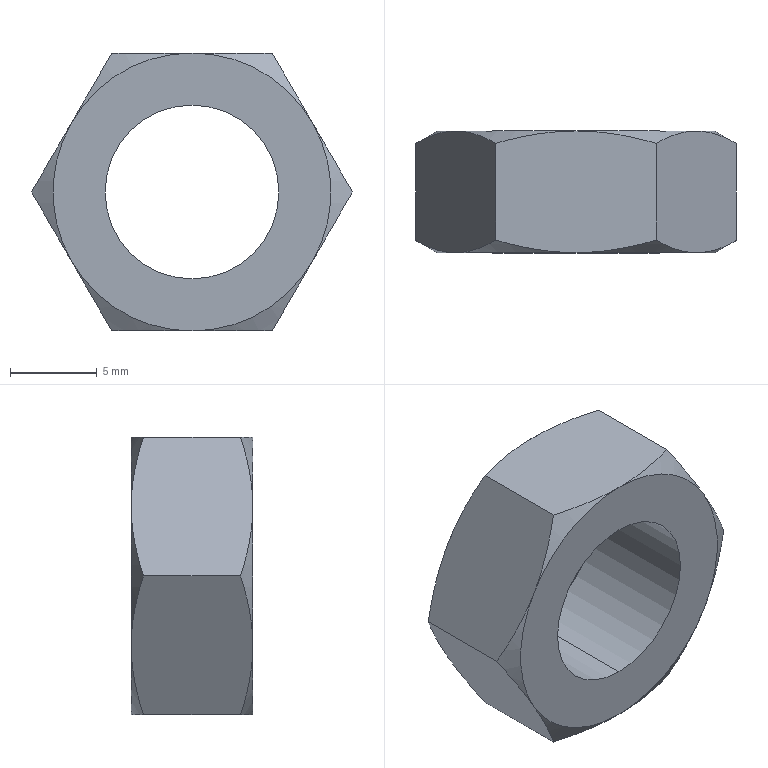Part | 1 solid | 22 faces | box 18.475 x 7 x 16 mm | volume 993.278 mm3 | cone 12 | plane 8 | cylinder 2 | commonest cylinder face diameters 10 x2
STEP:
#1=CARTESIAN_POINT('',(0.,7.,-5.));
#2=VERTEX_POINT('',#1);
#3=CARTESIAN_POINT('',(0.,7.,5.));
#4=VERTEX_POINT('',#3);
#5=CARTESIAN_POINT('',(0.,7.,0.));
#6=DIRECTION('',(0.,1.,0.));
#7=DIRECTION('',(0.,0.,1.));
#8=AXIS2_PLACEMENT_3D('',#5,#6,#7);
#9=CIRCLE('',#8,5.);
#10=EDGE_CURVE('',#2,#4,#9,.T.);
#11=ORIENTED_EDGE('',*,*,#10,.T.);
#12=CARTESIAN_POINT('',(0.,0.,5.));
#13=VERTEX_POINT('',#12);
#14=CARTESIAN_POINT('',(0.,7.,5.));
#15=DIRECTION('',(0.,-1.,0.));
#16=VECTOR('',#15,1000.);
#17=LINE('',#14,#16);
#18=EDGE_CURVE('',#4,#13,#17,.T.);
#19=ORIENTED_EDGE('',*,*,#18,.T.);
#20=CARTESIAN_POINT('',(0.,0.,-5.));
#21=VERTEX_POINT('',#20);
#22=CARTESIAN_POINT('',(0.,0.,0.));
#23=DIRECTION('',(0.,1.,0.));
#24=DIRECTION('',(0.,0.,1.));
#25=AXIS2_PLACEMENT_3D('',#22,#23,#24);
#26=CIRCLE('',#25,5.);
#27=EDGE_CURVE('',#21,#13,#26,.T.);
#28=ORIENTED_EDGE('',*,*,#27,.F.);
#29=CARTESIAN_POINT('',(0.,7.,-5.));
#30=DIRECTION('',(0.,-1.,0.));
#31=VECTOR('',#30,1000.);
#32=LINE('',#29,#31);
#33=EDGE_CURVE('',#2,#21,#32,.T.);
#34=ORIENTED_EDGE('',*,*,#33,.F.);
#35=EDGE_LOOP('',(#11,#19,#28,#34));
#36=FACE_OUTER_BOUND('',#35,.T.);
#37=CARTESIAN_POINT('',(0.,7.,0.));
#38=DIRECTION('',(0.,-1.,0.));
#39=DIRECTION('',(0.,0.,-1.));
#40=AXIS2_PLACEMENT_3D('',#37,#38,#39);
#41=CYLINDRICAL_SURFACE('',#40,5.);
#42=ADVANCED_FACE('',(#36),#41,.F.);
#43=CARTESIAN_POINT('',(9.238,0.7145,0.));
#44=VERTEX_POINT('',#43);
#45=CARTESIAN_POINT('',(6.928,0.,4.));
#46=VERTEX_POINT('',#45);
#47=CARTESIAN_POINT('',(9.238,0.7145,0.));
#48=CARTESIAN_POINT('',(9.041,0.6009,0.341));
#49=CARTESIAN_POINT('',(8.848,0.5005,0.6742));
#50=CARTESIAN_POINT('',(8.563,0.37,1.167));
#51=CARTESIAN_POINT('',(8.469,0.3298,1.331));
#52=CARTESIAN_POINT('',(8.328,0.2745,1.575));
#53=CARTESIAN_POINT('',(8.258,0.2482,1.696));
#54=CARTESIAN_POINT('',(8.188,0.2236,1.818));
#55=CARTESIAN_POINT('',(8.141,0.2077,1.899));
#56=CARTESIAN_POINT('',(8.119,0.2003,1.937));
#57=CARTESIAN_POINT('',(7.997,0.1609,2.148));
#58=CARTESIAN_POINT('',(7.901,0.1333,2.316));
#59=CARTESIAN_POINT('',(7.756,0.09752,2.567));
#60=CARTESIAN_POINT('',(7.708,0.08656,2.65));
#61=CARTESIAN_POINT('',(7.611,0.06657,2.817));
#62=CARTESIAN_POINT('',(7.564,0.05769,2.899));
#63=CARTESIAN_POINT('',(7.318,0.01648,3.325));
#64=CARTESIAN_POINT('',(7.124,0.,3.661));
#65=CARTESIAN_POINT('',(6.928,0.,4.));
#66=B_SPLINE_CURVE_WITH_KNOTS('',3,(#47,#48,#49,#50,#51,#52,#53,#54,#55,#56,#57,#58,#59,#60,#61,#62,#63,#64,#65),.UNSPECIFIED.,.F.,.F.,(4,2,2,1,2,2,2,2,2,4),(0.,0.25,0.375,0.4375,0.4687,0.5,0.625,0.6875,0.75,1.),.UNSPECIFIED.);
#67=EDGE_CURVE('',#44,#46,#66,.T.);
#68=ORIENTED_EDGE('',*,*,#67,.F.);
#69=CARTESIAN_POINT('',(9.238,6.285,0.));
#70=VERTEX_POINT('',#69);
#71=CARTESIAN_POINT('',(9.238,7.,0.));
#72=DIRECTION('',(0.,-1.,0.));
#73=VECTOR('',#72,1000.);
#74=LINE('',#71,#73);
#75=EDGE_CURVE('',#70,#44,#74,.T.);
#76=ORIENTED_EDGE('',*,*,#75,.F.);
#77=CARTESIAN_POINT('',(6.928,7.,4.));
#78=VERTEX_POINT('',#77);
#79=CARTESIAN_POINT('',(6.928,7.,4.));
#80=CARTESIAN_POINT('',(7.026,7.,3.83));
#81=CARTESIAN_POINT('',(7.124,6.996,3.661));
#82=CARTESIAN_POINT('',(7.271,6.983,3.407));
#83=CARTESIAN_POINT('',(7.319,6.978,3.322));
#84=CARTESIAN_POINT('',(7.417,6.966,3.153));
#85=CARTESIAN_POINT('',(7.468,6.959,3.066));
#86=CARTESIAN_POINT('',(7.612,6.934,2.815));
#87=CARTESIAN_POINT('',(7.708,6.914,2.648));
#88=CARTESIAN_POINT('',(7.853,6.878,2.397));
#89=CARTESIAN_POINT('',(7.926,6.859,2.272));
#90=CARTESIAN_POINT('',(7.999,6.837,2.146));
#91=CARTESIAN_POINT('',(8.047,6.823,2.061));
#92=CARTESIAN_POINT('',(8.073,6.815,2.017));
#93=CARTESIAN_POINT('',(8.469,6.686,1.331));
#94=CARTESIAN_POINT('',(8.844,6.512,0.6811));
#95=CARTESIAN_POINT('',(9.238,6.285,0.));
#96=B_SPLINE_CURVE_WITH_KNOTS('',3,(#79,#80,#81,#82,#83,#84,#85,#86,#87,#88,#89,#90,#91,#92,#93,#94,#95),.UNSPECIFIED.,.F.,.F.,(4,2,2,2,2,1,2,2,4),(0.,0.125,0.1875,0.25,0.375,0.4375,0.4687,0.5,1.),.UNSPECIFIED.);
#97=EDGE_CURVE('',#78,#70,#96,.T.);
#98=ORIENTED_EDGE('',*,*,#97,.F.);
#99=CARTESIAN_POINT('',(4.619,6.285,8.));
#100=VERTEX_POINT('',#99);
#101=CARTESIAN_POINT('',(4.619,6.285,8.));
#102=CARTESIAN_POINT('',(4.816,6.399,7.659));
#103=CARTESIAN_POINT('',(5.008,6.499,7.326));
#104=CARTESIAN_POINT('',(5.293,6.63,6.832));
#105=CARTESIAN_POINT('',(5.387,6.67,6.669));
#106=CARTESIAN_POINT('',(5.528,6.725,6.425));
#107=CARTESIAN_POINT('',(5.598,6.752,6.304));
#108=CARTESIAN_POINT('',(5.668,6.776,6.182));
#109=CARTESIAN_POINT('',(5.715,6.792,6.101));
#110=CARTESIAN_POINT('',(5.737,6.8,6.063));
#111=CARTESIAN_POINT('',(5.859,6.839,5.852));
#112=CARTESIAN_POINT('',(5.956,6.867,5.684));
#113=CARTESIAN_POINT('',(6.101,6.902,5.433));
#114=CARTESIAN_POINT('',(6.149,6.913,5.35));
#115=CARTESIAN_POINT('',(6.245,6.933,5.183));
#116=CARTESIAN_POINT('',(6.292,6.942,5.101));
#117=CARTESIAN_POINT('',(6.538,6.984,4.675));
#118=CARTESIAN_POINT('',(6.733,7.,4.339));
#119=CARTESIAN_POINT('',(6.928,7.,4.));
#120=B_SPLINE_CURVE_WITH_KNOTS('',3,(#101,#102,#103,#104,#105,#106,#107,#108,#109,#110,#111,#112,#113,#114,#115,#116,#117,#118,#119),.UNSPECIFIED.,.F.,.F.,(4,2,2,1,2,2,2,2,2,4),(0.,0.25,0.375,0.4375,0.4687,0.5,0.625,0.6875,0.75,1.),.UNSPECIFIED.);
#121=EDGE_CURVE('',#100,#78,#120,.T.);
#122=ORIENTED_EDGE('',*,*,#121,.F.);
#123=CARTESIAN_POINT('',(4.619,0.7145,8.));
#124=VERTEX_POINT('',#123);
#125=CARTESIAN_POINT('',(4.619,7.,8.));
#126=DIRECTION('',(0.,-1.,0.));
#127=VECTOR('',#126,1000.);
#128=LINE('',#125,#127);
#129=EDGE_CURVE('',#100,#124,#128,.T.);
#130=ORIENTED_EDGE('',*,*,#129,.T.);
#131=CARTESIAN_POINT('',(6.928,0.,4.));
#132=CARTESIAN_POINT('',(6.83,0.,4.17));
#133=CARTESIAN_POINT('',(6.732,0.004131,4.339));
#134=CARTESIAN_POINT('',(6.586,0.01652,4.593));
#135=CARTESIAN_POINT('',(6.537,0.02169,4.678));
#136=CARTESIAN_POINT('',(6.439,0.03408,4.847));
#137=CARTESIAN_POINT('',(6.389,0.04148,4.934));
#138=CARTESIAN_POINT('',(6.244,0.06575,5.185));
#139=CARTESIAN_POINT('',(6.148,0.08579,5.352));
#140=CARTESIAN_POINT('',(6.003,0.1216,5.603));
#141=CARTESIAN_POINT('',(5.93,0.141,5.728));
#142=CARTESIAN_POINT('',(5.858,0.1625,5.854));
#143=CARTESIAN_POINT('',(5.809,0.1773,5.939));
#144=CARTESIAN_POINT('',(5.784,0.1853,5.983));
#145=CARTESIAN_POINT('',(5.387,0.3136,6.669));
#146=CARTESIAN_POINT('',(5.012,0.4875,7.319));
#147=CARTESIAN_POINT('',(4.619,0.7145,8.));
#148=B_SPLINE_CURVE_WITH_KNOTS('',3,(#131,#132,#133,#134,#135,#136,#137,#138,#139,#140,#141,#142,#143,#144,#145,#146,#147),.UNSPECIFIED.,.F.,.F.,(4,2,2,2,2,1,2,2,4),(0.,0.125,0.1875,0.25,0.375,0.4375,0.4687,0.5,1.),.UNSPECIFIED.);
#149=EDGE_CURVE('',#46,#124,#148,.T.);
#150=ORIENTED_EDGE('',*,*,#149,.F.);
#151=EDGE_LOOP('',(#68,#76,#98,#122,#130,#150));
#152=FACE_OUTER_BOUND('',#151,.T.);
#153=CARTESIAN_POINT('',(4.619,7.,8.));
#154=DIRECTION('',(-0.866,0.,-0.5));
#155=DIRECTION('',(-0.5,0.,0.866));
#156=AXIS2_PLACEMENT_3D('',#153,#154,#155);
#157=PLANE('',#156);
#158=ADVANCED_FACE('',(#152),#157,.F.);
#159=CARTESIAN_POINT('',(4.619,0.7145,-8.));
#160=VERTEX_POINT('',#159);
#161=CARTESIAN_POINT('',(6.928,0.,-4.));
#162=VERTEX_POINT('',#161);
#163=CARTESIAN_POINT('',(4.619,0.7145,-8.));
#164=CARTESIAN_POINT('',(4.816,0.6009,-7.659));
#165=CARTESIAN_POINT('',(5.008,0.5005,-7.326));
#166=CARTESIAN_POINT('',(5.293,0.37,-6.832));
#167=CARTESIAN_POINT('',(5.387,0.3298,-6.669));
#168=CARTESIAN_POINT('',(5.528,0.2745,-6.425));
#169=CARTESIAN_POINT('',(5.598,0.2482,-6.304));
#170=CARTESIAN_POINT('',(5.668,0.2236,-6.182));
#171=CARTESIAN_POINT('',(5.715,0.2077,-6.101));
#172=CARTESIAN_POINT('',(5.737,0.2003,-6.063));
#173=CARTESIAN_POINT('',(5.859,0.1609,-5.852));
#174=CARTESIAN_POINT('',(5.956,0.1333,-5.684));
#175=CARTESIAN_POINT('',(6.101,0.09752,-5.433));
#176=CARTESIAN_POINT('',(6.149,0.08656,-5.35));
#177=CARTESIAN_POINT('',(6.245,0.06657,-5.183));
#178=CARTESIAN_POINT('',(6.292,0.05769,-5.101));
#179=CARTESIAN_POINT('',(6.538,0.01648,-4.675));
#180=CARTESIAN_POINT('',(6.733,0.,-4.339));
#181=CARTESIAN_POINT('',(6.928,0.,-4.));
#182=B_SPLINE_CURVE_WITH_KNOTS('',3,(#163,#164,#165,#166,#167,#168,#169,#170,#171,#172,#173,#174,#175,#176,#177,#178,#179,#180,#181),.UNSPECIFIED.,.F.,.F.,(4,2,2,1,2,2,2,2,2,4),(0.,0.25,0.375,0.4375,0.4687,0.5,0.625,0.6875,0.75,1.),.UNSPECIFIED.);
#183=EDGE_CURVE('',#160,#162,#182,.T.);
#184=ORIENTED_EDGE('',*,*,#183,.F.);
#185=CARTESIAN_POINT('',(4.619,6.285,-8.));
#186=VERTEX_POINT('',#185);
#187=CARTESIAN_POINT('',(4.619,7.,-8.));
#188=DIRECTION('',(0.,-1.,0.));
#189=VECTOR('',#188,1000.);
#190=LINE('',#187,#189);
#191=EDGE_CURVE('',#186,#160,#190,.T.);
#192=ORIENTED_EDGE('',*,*,#191,.F.);
#193=CARTESIAN_POINT('',(6.928,7.,-4.));
#194=VERTEX_POINT('',#193);
#195=CARTESIAN_POINT('',(6.928,7.,-4.));
#196=CARTESIAN_POINT('',(6.83,7.,-4.17));
#197=CARTESIAN_POINT('',(6.732,6.996,-4.339));
#198=CARTESIAN_POINT('',(6.586,6.983,-4.593));
#199=CARTESIAN_POINT('',(6.537,6.978,-4.678));
#200=CARTESIAN_POINT('',(6.439,6.966,-4.847));
#201=CARTESIAN_POINT('',(6.389,6.959,-4.934));
#202=CARTESIAN_POINT('',(6.244,6.934,-5.185));
#203=CARTESIAN_POINT('',(6.148,6.914,-5.352));
#204=CARTESIAN_POINT('',(6.003,6.878,-5.603));
#205=CARTESIAN_POINT('',(5.93,6.859,-5.728));
#206=CARTESIAN_POINT('',(5.858,6.837,-5.854));
#207=CARTESIAN_POINT('',(5.809,6.823,-5.939));
#208=CARTESIAN_POINT('',(5.784,6.815,-5.983));
#209=CARTESIAN_POINT('',(5.387,6.686,-6.669));
#210=CARTESIAN_POINT('',(5.012,6.512,-7.319));
#211=CARTESIAN_POINT('',(4.619,6.285,-8.));
#212=B_SPLINE_CURVE_WITH_KNOTS('',3,(#195,#196,#197,#198,#199,#200,#201,#202,#203,#204,#205,#206,#207,#208,#209,#210,#211),.UNSPECIFIED.,.F.,.F.,(4,2,2,2,2,1,2,2,4),(0.,0.125,0.1875,0.25,0.375,0.4375,0.4688,0.5,1.),.UNSPECIFIED.);
#213=EDGE_CURVE('',#194,#186,#212,.T.);
#214=ORIENTED_EDGE('',*,*,#213,.F.);
#215=CARTESIAN_POINT('',(9.238,6.285,0.));
#216=CARTESIAN_POINT('',(9.041,6.399,-0.341));
#217=CARTESIAN_POINT('',(8.848,6.499,-0.6742));
#218=CARTESIAN_POINT('',(8.563,6.63,-1.167));
#219=CARTESIAN_POINT('',(8.469,6.67,-1.331));
#220=CARTESIAN_POINT('',(8.328,6.725,-1.575));
#221=CARTESIAN_POINT('',(8.258,6.752,-1.696));
#222=CARTESIAN_POINT('',(8.188,6.776,-1.818));
#223=CARTESIAN_POINT('',(8.141,6.792,-1.899));
#224=CARTESIAN_POINT('',(8.119,6.8,-1.937));
#225=CARTESIAN_POINT('',(7.997,6.839,-2.148));
#226=CARTESIAN_POINT('',(7.901,6.867,-2.316));
#227=CARTESIAN_POINT('',(7.756,6.902,-2.567));
#228=CARTESIAN_POINT('',(7.708,6.913,-2.65));
#229=CARTESIAN_POINT('',(7.611,6.933,-2.817));
#230=CARTESIAN_POINT('',(7.564,6.942,-2.899));
#231=CARTESIAN_POINT('',(7.318,6.984,-3.325));
#232=CARTESIAN_POINT('',(7.124,7.,-3.661));
#233=CARTESIAN_POINT('',(6.928,7.,-4.));
#234=B_SPLINE_CURVE_WITH_KNOTS('',3,(#215,#216,#217,#218,#219,#220,#221,#222,#223,#224,#225,#226,#227,#228,#229,#230,#231,#232,#233),.UNSPECIFIED.,.F.,.F.,(4,2,2,1,2,2,2,2,2,4),(0.,0.25,0.375,0.4375,0.4687,0.5,0.625,0.6875,0.75,1.),.UNSPECIFIED.);
#235=EDGE_CURVE('',#70,#194,#234,.T.);
#236=ORIENTED_EDGE('',*,*,#235,.F.);
#237=ORIENTED_EDGE('',*,*,#75,.T.);
#238=CARTESIAN_POINT('',(6.928,0.,-4.));
#239=CARTESIAN_POINT('',(7.026,0.,-3.83));
#240=CARTESIAN_POINT('',(7.124,0.004131,-3.661));
#241=CARTESIAN_POINT('',(7.271,0.01652,-3.407));
#242=CARTESIAN_POINT('',(7.319,0.02169,-3.322));
#243=CARTESIAN_POINT('',(7.417,0.03408,-3.153));
#244=CARTESIAN_POINT('',(7.468,0.04148,-3.066));
#245=CARTESIAN_POINT('',(7.612,0.06575,-2.815));
#246=CARTESIAN_POINT('',(7.708,0.08579,-2.648));
#247=CARTESIAN_POINT('',(7.853,0.1216,-2.397));
#248=CARTESIAN_POINT('',(7.926,0.141,-2.272));
#249=CARTESIAN_POINT('',(7.999,0.1625,-2.146));
#250=CARTESIAN_POINT('',(8.047,0.1773,-2.061));
#251=CARTESIAN_POINT('',(8.073,0.1853,-2.017));
#252=CARTESIAN_POINT('',(8.469,0.3136,-1.331));
#253=CARTESIAN_POINT('',(8.844,0.4875,-0.6811));
#254=CARTESIAN_POINT('',(9.238,0.7145,0.));
#255=B_SPLINE_CURVE_WITH_KNOTS('',3,(#238,#239,#240,#241,#242,#243,#244,#245,#246,#247,#248,#249,#250,#251,#252,#253,#254),.UNSPECIFIED.,.F.,.F.,(4,2,2,2,2,1,2,2,4),(0.,0.125,0.1875,0.25,0.375,0.4375,0.4688,0.5,1.),.UNSPECIFIED.);
#256=EDGE_CURVE('',#162,#44,#255,.T.);
#257=ORIENTED_EDGE('',*,*,#256,.F.);
#258=EDGE_LOOP('',(#184,#192,#214,#236,#237,#257));
#259=FACE_OUTER_BOUND('',#258,.T.);
#260=CARTESIAN_POINT('',(9.238,7.,0.));
#261=DIRECTION('',(-0.866,0.,0.5));
#262=DIRECTION('',(0.,1.,0.));
#263=AXIS2_PLACEMENT_3D('',#260,#261,#262);
#264=PLANE('',#263);
#265=ADVANCED_FACE('',(#259),#264,.F.);
#266=CARTESIAN_POINT('',(-4.619,0.7145,-8.));
#267=VERTEX_POINT('',#266);
#268=CARTESIAN_POINT('',(0.,0.,-8.));
#269=VERTEX_POINT('',#268);
#270=CARTESIAN_POINT('',(-4.619,0.7145,-8.));
#271=CARTESIAN_POINT('',(-4.224,0.6006,-8.));
#272=CARTESIAN_POINT('',(-3.838,0.5,-8.));
#273=CARTESIAN_POINT('',(-3.267,0.3692,-8.));
#274=CARTESIAN_POINT('',(-3.078,0.329,-8.));
#275=CARTESIAN_POINT('',(-2.796,0.2737,-8.));
#276=CARTESIAN_POINT('',(-2.655,0.2472,-8.));
#277=CARTESIAN_POINT('',(-2.515,0.2227,-8.));
#278=CARTESIAN_POINT('',(-2.421,0.2068,-8.));
#279=CARTESIAN_POINT('',(-2.376,0.1993,-8.));
#280=CARTESIAN_POINT('',(-2.132,0.1601,-8.));
#281=CARTESIAN_POINT('',(-1.939,0.1325,-8.));
#282=CARTESIAN_POINT('',(-1.65,0.09686,-8.));
#283=CARTESIAN_POINT('',(-1.553,0.08594,-8.));
#284=CARTESIAN_POINT('',(-1.36,0.06602,-8.));
#285=CARTESIAN_POINT('',(-1.266,0.05715,-8.));
#286=CARTESIAN_POINT('',(-0.776,0.01633,-8.));
#287=CARTESIAN_POINT('',(-0.3895,0.,-8.));
#288=CARTESIAN_POINT('',(0.,0.,-8.));
#289=B_SPLINE_CURVE_WITH_KNOTS('',3,(#270,#271,#272,#273,#274,#275,#276,#277,#278,#279,#280,#281,#282,#283,#284,#285,#286,#287,#288),.UNSPECIFIED.,.F.,.F.,(4,2,2,1,2,2,2,2,2,4),(0.,0.25,0.375,0.4375,0.4687,0.5,0.625,0.6875,0.75,1.),.UNSPECIFIED.);
#290=EDGE_CURVE('',#267,#269,#289,.T.);
#291=ORIENTED_EDGE('',*,*,#290,.F.);
#292=CARTESIAN_POINT('',(-4.619,6.285,-8.));
#293=VERTEX_POINT('',#292);
#294=CARTESIAN_POINT('',(-4.619,7.,-8.));
#295=DIRECTION('',(0.,-1.,0.));
#296=VECTOR('',#295,1000.);
#297=LINE('',#294,#296);
#298=EDGE_CURVE('',#293,#267,#297,.T.);
#299=ORIENTED_EDGE('',*,*,#298,.F.);
#300=CARTESIAN_POINT('',(0.,7.,-8.));
#301=VERTEX_POINT('',#300);
#302=CARTESIAN_POINT('',(0.,7.,-8.));
#303=CARTESIAN_POINT('',(-0.1947,7.,-8.));
#304=CARTESIAN_POINT('',(-0.3887,6.996,-8.));
#305=CARTESIAN_POINT('',(-0.6801,6.984,-8.));
#306=CARTESIAN_POINT('',(-0.7773,6.979,-8.));
#307=CARTESIAN_POINT('',(-0.9721,6.966,-8.));
#308=CARTESIAN_POINT('',(-1.071,6.959,-8.));
#309=CARTESIAN_POINT('',(-1.36,6.935,-8.));
#310=CARTESIAN_POINT('',(-1.553,6.915,-8.));
#311=CARTESIAN_POINT('',(-1.842,6.879,-8.));
#312=CARTESIAN_POINT('',(-1.987,6.86,-8.));
#313=CARTESIAN_POINT('',(-2.133,6.839,-8.));
#314=CARTESIAN_POINT('',(-2.23,6.824,-8.));
#315=CARTESIAN_POINT('',(-2.28,6.816,-8.));
#316=CARTESIAN_POINT('',(-3.076,6.688,-8.));
#317=CARTESIAN_POINT('',(-3.829,6.513,-8.));
#318=CARTESIAN_POINT('',(-4.619,6.285,-8.));
#319=B_SPLINE_CURVE_WITH_KNOTS('',3,(#302,#303,#304,#305,#306,#307,#308,#309,#310,#311,#312,#313,#314,#315,#316,#317,#318),.UNSPECIFIED.,.F.,.F.,(4,2,2,2,2,1,2,2,4),(0.,0.125,0.1875,0.25,0.375,0.4375,0.4687,0.5,1.),.UNSPECIFIED.);
#320=EDGE_CURVE('',#301,#293,#319,.T.);
#321=ORIENTED_EDGE('',*,*,#320,.F.);
#322=CARTESIAN_POINT('',(4.619,6.285,-8.));
#323=CARTESIAN_POINT('',(4.227,6.399,-8.));
#324=CARTESIAN_POINT('',(3.844,6.498,-8.));
#325=CARTESIAN_POINT('',(3.277,6.629,-8.));
#326=CARTESIAN_POINT('',(3.09,6.669,-8.));
#327=CARTESIAN_POINT('',(2.81,6.724,-8.));
#328=CARTESIAN_POINT('',(2.67,6.75,-8.));
#329=CARTESIAN_POINT('',(2.507,6.779,-8.));
#330=CARTESIAN_POINT('',(2.437,6.79,-8.));
#331=CARTESIAN_POINT('',(2.391,6.798,-8.));
#332=CARTESIAN_POINT('',(2.369,6.802,-8.));
#333=CARTESIAN_POINT('',(2.149,6.838,-8.));
#334=CARTESIAN_POINT('',(1.954,6.865,-8.));
#335=CARTESIAN_POINT('',(1.662,6.902,-8.));
#336=CARTESIAN_POINT('',(1.565,6.913,-8.));
#337=CARTESIAN_POINT('',(1.371,6.933,-8.));
#338=CARTESIAN_POINT('',(1.275,6.942,-8.));
#339=CARTESIAN_POINT('',(0.7811,6.983,-8.));
#340=CARTESIAN_POINT('',(0.3917,7.,-8.));
#341=CARTESIAN_POINT('',(0.,7.,-8.));
#342=B_SPLINE_CURVE_WITH_KNOTS('',3,(#322,#323,#324,#325,#326,#327,#328,#329,#330,#331,#332,#333,#334,#335,#336,#337,#338,#339,#340,#341),.UNSPECIFIED.,.F.,.F.,(4,2,2,1,1,2,2,2,2,2,4),(0.,0.25,0.375,0.4375,0.4688,0.4844,0.5,0.625,0.6875,0.75,1.),.UNSPECIFIED.);
#343=EDGE_CURVE('',#186,#301,#342,.T.);
#344=ORIENTED_EDGE('',*,*,#343,.F.);
#345=ORIENTED_EDGE('',*,*,#191,.T.);
#346=CARTESIAN_POINT('',(0.,0.,-8.));
#347=CARTESIAN_POINT('',(0.1958,0.,-8.));
#348=CARTESIAN_POINT('',(0.3911,0.00415,-8.));
#349=CARTESIAN_POINT('',(0.6847,0.0166,-8.));
#350=CARTESIAN_POINT('',(0.7826,0.02179,-8.));
#351=CARTESIAN_POINT('',(0.9791,0.03423,-8.));
#352=CARTESIAN_POINT('',(1.079,0.04163,-8.));
#353=CARTESIAN_POINT('',(1.371,0.06613,-8.));
#354=CARTESIAN_POINT('',(1.565,0.08634,-8.));
#355=CARTESIAN_POINT('',(1.857,0.1225,-8.));
#356=CARTESIAN_POINT('',(2.002,0.142,-8.));
#357=CARTESIAN_POINT('',(2.173,0.1673,-8.));
#358=CARTESIAN_POINT('',(2.247,0.1786,-8.));
#359=CARTESIAN_POINT('',(2.295,0.1864,-8.));
#360=CARTESIAN_POINT('',(2.321,0.1905,-8.));
#361=CARTESIAN_POINT('',(3.088,0.3149,-8.));
#362=CARTESIAN_POINT('',(3.835,0.4884,-8.));
#363=CARTESIAN_POINT('',(4.619,0.7145,-8.));
#364=B_SPLINE_CURVE_WITH_KNOTS('',3,(#346,#347,#348,#349,#350,#351,#352,#353,#354,#355,#356,#357,#358,#359,#360,#361,#362,#363),.UNSPECIFIED.,.F.,.F.,(4,2,2,2,2,1,1,2,2,4),(0.,0.125,0.1875,0.25,0.375,0.4375,0.4688,0.4844,0.5,1.),.UNSPECIFIED.);
#365=EDGE_CURVE('',#269,#160,#364,.T.);
#366=ORIENTED_EDGE('',*,*,#365,.F.);
#367=EDGE_LOOP('',(#291,#299,#321,#344,#345,#366));
#368=FACE_OUTER_BOUND('',#367,.T.);
#369=CARTESIAN_POINT('',(4.619,7.,-8.));
#370=DIRECTION('',(0.,0.,1.));
#371=DIRECTION('',(1.,0.,0.));
#372=AXIS2_PLACEMENT_3D('',#369,#370,#371);
#373=PLANE('',#372);
#374=ADVANCED_FACE('',(#368),#373,.F.);
#375=CARTESIAN_POINT('',(-9.238,0.7145,0.));
#376=VERTEX_POINT('',#375);
#377=CARTESIAN_POINT('',(-6.928,0.,-4.));
#378=VERTEX_POINT('',#377);
#379=CARTESIAN_POINT('',(-9.238,0.7145,0.));
#380=CARTESIAN_POINT('',(-9.041,0.6009,-0.341));
#381=CARTESIAN_POINT('',(-8.848,0.5005,-0.6742));
#382=CARTESIAN_POINT('',(-8.563,0.37,-1.167));
#383=CARTESIAN_POINT('',(-8.469,0.3298,-1.331));
#384=CARTESIAN_POINT('',(-8.328,0.2745,-1.575));
#385=CARTESIAN_POINT('',(-8.258,0.2482,-1.696));
#386=CARTESIAN_POINT('',(-8.188,0.2236,-1.818));
#387=CARTESIAN_POINT('',(-8.141,0.2077,-1.899));
#388=CARTESIAN_POINT('',(-8.119,0.2003,-1.937));
#389=CARTESIAN_POINT('',(-7.997,0.1609,-2.148));
#390=CARTESIAN_POINT('',(-7.901,0.1333,-2.316));
#391=CARTESIAN_POINT('',(-7.756,0.09752,-2.567));
#392=CARTESIAN_POINT('',(-7.708,0.08656,-2.65));
#393=CARTESIAN_POINT('',(-7.611,0.06657,-2.817));
#394=CARTESIAN_POINT('',(-7.564,0.05769,-2.899));
#395=CARTESIAN_POINT('',(-7.318,0.01648,-3.325));
#396=CARTESIAN_POINT('',(-7.124,0.,-3.661));
#397=CARTESIAN_POINT('',(-6.928,0.,-4.));
#398=B_SPLINE_CURVE_WITH_KNOTS('',3,(#379,#380,#381,#382,#383,#384,#385,#386,#387,#388,#389,#390,#391,#392,#393,#394,#395,#396,#397),.UNSPECIFIED.,.F.,.F.,(4,2,2,1,2,2,2,2,2,4),(0.,0.25,0.375,0.4375,0.4688,0.5,0.625,0.6875,0.75,1.),.UNSPECIFIED.);
#399=EDGE_CURVE('',#376,#378,#398,.T.);
#400=ORIENTED_EDGE('',*,*,#399,.F.);
#401=CARTESIAN_POINT('',(-9.238,6.285,0.));
#402=VERTEX_POINT('',#401);
#403=CARTESIAN_POINT('',(-9.238,7.,0.));
#404=DIRECTION('',(0.,-1.,0.));
#405=VECTOR('',#404,1000.);
#406=LINE('',#403,#405);
#407=EDGE_CURVE('',#402,#376,#406,.T.);
#408=ORIENTED_EDGE('',*,*,#407,.F.);
#409=CARTESIAN_POINT('',(-6.928,7.,-4.));
#410=VERTEX_POINT('',#409);
#411=CARTESIAN_POINT('',(-6.928,7.,-4.));
#412=CARTESIAN_POINT('',(-7.026,7.,-3.83));
#413=CARTESIAN_POINT('',(-7.124,6.996,-3.661));
#414=CARTESIAN_POINT('',(-7.271,6.983,-3.407));
#415=CARTESIAN_POINT('',(-7.319,6.978,-3.322));
#416=CARTESIAN_POINT('',(-7.417,6.966,-3.153));
#417=CARTESIAN_POINT('',(-7.468,6.959,-3.066));
#418=CARTESIAN_POINT('',(-7.612,6.934,-2.815));
#419=CARTESIAN_POINT('',(-7.708,6.914,-2.648));
#420=CARTESIAN_POINT('',(-7.853,6.878,-2.397));
#421=CARTESIAN_POINT('',(-7.926,6.859,-2.272));
#422=CARTESIAN_POINT('',(-7.999,6.837,-2.146));
#423=CARTESIAN_POINT('',(-8.047,6.823,-2.061));
#424=CARTESIAN_POINT('',(-8.073,6.815,-2.017));
#425=CARTESIAN_POINT('',(-8.469,6.686,-1.331));
#426=CARTESIAN_POINT('',(-8.844,6.512,-0.6811));
#427=CARTESIAN_POINT('',(-9.238,6.285,0.));
#428=B_SPLINE_CURVE_WITH_KNOTS('',3,(#411,#412,#413,#414,#415,#416,#417,#418,#419,#420,#421,#422,#423,#424,#425,#426,#427),.UNSPECIFIED.,.F.,.F.,(4,2,2,2,2,1,2,2,4),(0.,0.125,0.1875,0.25,0.375,0.4375,0.4687,0.5,1.),.UNSPECIFIED.);
#429=EDGE_CURVE('',#410,#402,#428,.T.);
#430=ORIENTED_EDGE('',*,*,#429,.F.);
#431=CARTESIAN_POINT('',(-4.619,6.285,-8.));
#432=CARTESIAN_POINT('',(-4.816,6.399,-7.659));
#433=CARTESIAN_POINT('',(-5.008,6.499,-7.326));
#434=CARTESIAN_POINT('',(-5.293,6.63,-6.832));
#435=CARTESIAN_POINT('',(-5.387,6.67,-6.669));
#436=CARTESIAN_POINT('',(-5.528,6.725,-6.425));
#437=CARTESIAN_POINT('',(-5.598,6.752,-6.304));
#438=CARTESIAN_POINT('',(-5.668,6.776,-6.182));
#439=CARTESIAN_POINT('',(-5.715,6.792,-6.101));
#440=CARTESIAN_POINT('',(-5.737,6.8,-6.063));
#441=CARTESIAN_POINT('',(-5.859,6.839,-5.852));
#442=CARTESIAN_POINT('',(-5.956,6.867,-5.684));
#443=CARTESIAN_POINT('',(-6.101,6.902,-5.433));
#444=CARTESIAN_POINT('',(-6.149,6.913,-5.35));
#445=CARTESIAN_POINT('',(-6.245,6.933,-5.183));
#446=CARTESIAN_POINT('',(-6.292,6.942,-5.101));
#447=CARTESIAN_POINT('',(-6.538,6.984,-4.675));
#448=CARTESIAN_POINT('',(-6.733,7.,-4.339));
#449=CARTESIAN_POINT('',(-6.928,7.,-4.));
#450=B_SPLINE_CURVE_WITH_KNOTS('',3,(#431,#432,#433,#434,#435,#436,#437,#438,#439,#440,#441,#442,#443,#444,#445,#446,#447,#448,#449),.UNSPECIFIED.,.F.,.F.,(4,2,2,1,2,2,2,2,2,4),(0.,0.25,0.375,0.4375,0.4688,0.5,0.625,0.6875,0.75,1.),.UNSPECIFIED.);
#451=EDGE_CURVE('',#293,#410,#450,.T.);
#452=ORIENTED_EDGE('',*,*,#451,.F.);
#453=ORIENTED_EDGE('',*,*,#298,.T.);
#454=CARTESIAN_POINT('',(-6.928,0.,-4.));
#455=CARTESIAN_POINT('',(-6.83,0.,-4.17));
#456=CARTESIAN_POINT('',(-6.732,0.004131,-4.339));
#457=CARTESIAN_POINT('',(-6.586,0.01652,-4.593));
#458=CARTESIAN_POINT('',(-6.537,0.02169,-4.678));
#459=CARTESIAN_POINT('',(-6.439,0.03408,-4.847));
#460=CARTESIAN_POINT('',(-6.389,0.04148,-4.934));
#461=CARTESIAN_POINT('',(-6.244,0.06575,-5.185));
#462=CARTESIAN_POINT('',(-6.148,0.08579,-5.352));
#463=CARTESIAN_POINT('',(-6.003,0.1216,-5.603));
#464=CARTESIAN_POINT('',(-5.93,0.141,-5.728));
#465=CARTESIAN_POINT('',(-5.858,0.1625,-5.854));
#466=CARTESIAN_POINT('',(-5.809,0.1773,-5.939));
#467=CARTESIAN_POINT('',(-5.784,0.1853,-5.983));
#468=CARTESIAN_POINT('',(-5.387,0.3136,-6.669));
#469=CARTESIAN_POINT('',(-5.012,0.4875,-7.319));
#470=CARTESIAN_POINT('',(-4.619,0.7145,-8.));
#471=B_SPLINE_CURVE_WITH_KNOTS('',3,(#454,#455,#456,#457,#458,#459,#460,#461,#462,#463,#464,#465,#466,#467,#468,#469,#470),.UNSPECIFIED.,.F.,.F.,(4,2,2,2,2,1,2,2,4),(0.,0.125,0.1875,0.25,0.375,0.4375,0.4687,0.5,1.),.UNSPECIFIED.);
#472=EDGE_CURVE('',#378,#267,#471,.T.);
#473=ORIENTED_EDGE('',*,*,#472,.F.);
#474=EDGE_LOOP('',(#400,#408,#430,#452,#453,#473));
#475=FACE_OUTER_BOUND('',#474,.T.);
#476=CARTESIAN_POINT('',(-4.619,7.,-8.));
#477=DIRECTION('',(0.866,0.,0.5));
#478=DIRECTION('',(0.,-1.,0.));
#479=AXIS2_PLACEMENT_3D('',#476,#477,#478);
#480=PLANE('',#479);
#481=ADVANCED_FACE('',(#475),#480,.F.);
#482=CARTESIAN_POINT('',(-4.619,0.7145,8.));
#483=VERTEX_POINT('',#482);
#484=CARTESIAN_POINT('',(-6.928,0.,4.));
#485=VERTEX_POINT('',#484);
#486=CARTESIAN_POINT('',(-4.619,0.7145,8.));
#487=CARTESIAN_POINT('',(-4.816,0.6009,7.659));
#488=CARTESIAN_POINT('',(-5.008,0.5005,7.326));
#489=CARTESIAN_POINT('',(-5.293,0.37,6.832));
#490=CARTESIAN_POINT('',(-5.387,0.3298,6.669));
#491=CARTESIAN_POINT('',(-5.528,0.2745,6.425));
#492=CARTESIAN_POINT('',(-5.598,0.2482,6.304));
#493=CARTESIAN_POINT('',(-5.668,0.2236,6.182));
#494=CARTESIAN_POINT('',(-5.715,0.2077,6.101));
#495=CARTESIAN_POINT('',(-5.737,0.2003,6.063));
#496=CARTESIAN_POINT('',(-5.859,0.1609,5.852));
#497=CARTESIAN_POINT('',(-5.956,0.1333,5.684));
#498=CARTESIAN_POINT('',(-6.101,0.09752,5.433));
#499=CARTESIAN_POINT('',(-6.149,0.08656,5.35));
#500=CARTESIAN_POINT('',(-6.245,0.06657,5.183));
#501=CARTESIAN_POINT('',(-6.292,0.05769,5.101));
#502=CARTESIAN_POINT('',(-6.538,0.01648,4.675));
#503=CARTESIAN_POINT('',(-6.733,0.,4.339));
#504=CARTESIAN_POINT('',(-6.928,0.,4.));
#505=B_SPLINE_CURVE_WITH_KNOTS('',3,(#486,#487,#488,#489,#490,#491,#492,#493,#494,#495,#496,#497,#498,#499,#500,#501,#502,#503,#504),.UNSPECIFIED.,.F.,.F.,(4,2,2,1,2,2,2,2,2,4),(0.,0.25,0.375,0.4375,0.4688,0.5,0.625,0.6875,0.75,1.),.UNSPECIFIED.);
#506=EDGE_CURVE('',#483,#485,#505,.T.);
#507=ORIENTED_EDGE('',*,*,#506,.F.);
#508=CARTESIAN_POINT('',(-4.619,6.285,8.));
#509=VERTEX_POINT('',#508);
#510=CARTESIAN_POINT('',(-4.619,7.,8.));
#511=DIRECTION('',(0.,-1.,0.));
#512=VECTOR('',#511,1000.);
#513=LINE('',#510,#512);
#514=EDGE_CURVE('',#509,#483,#513,.T.);
#515=ORIENTED_EDGE('',*,*,#514,.F.);
#516=CARTESIAN_POINT('',(-6.928,7.,4.));
#517=VERTEX_POINT('',#516);
#518=CARTESIAN_POINT('',(-6.928,7.,4.));
#519=CARTESIAN_POINT('',(-6.83,7.,4.17));
#520=CARTESIAN_POINT('',(-6.732,6.996,4.339));
#521=CARTESIAN_POINT('',(-6.586,6.983,4.593));
#522=CARTESIAN_POINT('',(-6.537,6.978,4.678));
#523=CARTESIAN_POINT('',(-6.439,6.966,4.847));
#524=CARTESIAN_POINT('',(-6.389,6.959,4.934));
#525=CARTESIAN_POINT('',(-6.244,6.934,5.185));
#526=CARTESIAN_POINT('',(-6.148,6.914,5.352));
#527=CARTESIAN_POINT('',(-6.003,6.878,5.603));
#528=CARTESIAN_POINT('',(-5.93,6.859,5.728));
#529=CARTESIAN_POINT('',(-5.858,6.837,5.854));
#530=CARTESIAN_POINT('',(-5.809,6.823,5.939));
#531=CARTESIAN_POINT('',(-5.784,6.815,5.983));
#532=CARTESIAN_POINT('',(-5.387,6.686,6.669));
#533=CARTESIAN_POINT('',(-5.012,6.512,7.319));
#534=CARTESIAN_POINT('',(-4.619,6.285,8.));
#535=B_SPLINE_CURVE_WITH_KNOTS('',3,(#518,#519,#520,#521,#522,#523,#524,#525,#526,#527,#528,#529,#530,#531,#532,#533,#534),.UNSPECIFIED.,.F.,.F.,(4,2,2,2,2,1,2,2,4),(0.,0.125,0.1875,0.25,0.375,0.4375,0.4687,0.5,1.),.UNSPECIFIED.);
#536=EDGE_CURVE('',#517,#509,#535,.T.);
#537=ORIENTED_EDGE('',*,*,#536,.F.);
#538=CARTESIAN_POINT('',(-9.238,6.285,0.));
#539=CARTESIAN_POINT('',(-9.041,6.399,0.341));
#540=CARTESIAN_POINT('',(-8.848,6.499,0.6742));
#541=CARTESIAN_POINT('',(-8.563,6.63,1.167));
#542=CARTESIAN_POINT('',(-8.469,6.67,1.331));
#543=CARTESIAN_POINT('',(-8.328,6.725,1.575));
#544=CARTESIAN_POINT('',(-8.258,6.752,1.696));
#545=CARTESIAN_POINT('',(-8.188,6.776,1.818));
#546=CARTESIAN_POINT('',(-8.141,6.792,1.899));
#547=CARTESIAN_POINT('',(-8.119,6.8,1.937));
#548=CARTESIAN_POINT('',(-7.997,6.839,2.148));
#549=CARTESIAN_POINT('',(-7.901,6.867,2.316));
#550=CARTESIAN_POINT('',(-7.756,6.902,2.567));
#551=CARTESIAN_POINT('',(-7.708,6.913,2.65));
#552=CARTESIAN_POINT('',(-7.611,6.933,2.817));
#553=CARTESIAN_POINT('',(-7.564,6.942,2.899));
#554=CARTESIAN_POINT('',(-7.318,6.984,3.325));
#555=CARTESIAN_POINT('',(-7.124,7.,3.661));
#556=CARTESIAN_POINT('',(-6.928,7.,4.));
#557=B_SPLINE_CURVE_WITH_KNOTS('',3,(#538,#539,#540,#541,#542,#543,#544,#545,#546,#547,#548,#549,#550,#551,#552,#553,#554,#555,#556),.UNSPECIFIED.,.F.,.F.,(4,2,2,1,2,2,2,2,2,4),(0.,0.25,0.375,0.4375,0.4687,0.5,0.625,0.6875,0.75,1.),.UNSPECIFIED.);
#558=EDGE_CURVE('',#402,#517,#557,.T.);
#559=ORIENTED_EDGE('',*,*,#558,.F.);
#560=ORIENTED_EDGE('',*,*,#407,.T.);
#561=CARTESIAN_POINT('',(-6.928,0.,4.));
#562=CARTESIAN_POINT('',(-7.026,0.,3.83));
#563=CARTESIAN_POINT('',(-7.124,0.004131,3.661));
#564=CARTESIAN_POINT('',(-7.271,0.01652,3.407));
#565=CARTESIAN_POINT('',(-7.319,0.02169,3.322));
#566=CARTESIAN_POINT('',(-7.417,0.03408,3.153));
#567=CARTESIAN_POINT('',(-7.468,0.04148,3.066));
#568=CARTESIAN_POINT('',(-7.612,0.06575,2.815));
#569=CARTESIAN_POINT('',(-7.708,0.08579,2.648));
#570=CARTESIAN_POINT('',(-7.853,0.1216,2.397));
#571=CARTESIAN_POINT('',(-7.926,0.141,2.272));
#572=CARTESIAN_POINT('',(-7.999,0.1625,2.146));
#573=CARTESIAN_POINT('',(-8.047,0.1773,2.061));
#574=CARTESIAN_POINT('',(-8.073,0.1853,2.017));
#575=CARTESIAN_POINT('',(-8.469,0.3136,1.331));
#576=CARTESIAN_POINT('',(-8.844,0.4875,0.6811));
#577=CARTESIAN_POINT('',(-9.238,0.7145,0.));
#578=B_SPLINE_CURVE_WITH_KNOTS('',3,(#561,#562,#563,#564,#565,#566,#567,#568,#569,#570,#571,#572,#573,#574,#575,#576,#577),.UNSPECIFIED.,.F.,.F.,(4,2,2,2,2,1,2,2,4),(0.,0.125,0.1875,0.25,0.375,0.4375,0.4688,0.5,1.),.UNSPECIFIED.);
#579=EDGE_CURVE('',#485,#376,#578,.T.);
#580=ORIENTED_EDGE('',*,*,#579,.F.);
#581=EDGE_LOOP('',(#507,#515,#537,#559,#560,#580));
#582=FACE_OUTER_BOUND('',#581,.T.);
#583=CARTESIAN_POINT('',(-9.238,7.,0.));
#584=DIRECTION('',(0.866,0.,-0.5));
#585=DIRECTION('',(0.,-1.,0.));
#586=AXIS2_PLACEMENT_3D('',#583,#584,#585);
#587=PLANE('',#586);
#588=ADVANCED_FACE('',(#582),#587,.F.);
#589=CARTESIAN_POINT('',(0.,0.,8.));
#590=VERTEX_POINT('',#589);
#591=CARTESIAN_POINT('',(4.619,0.7145,8.));
#592=CARTESIAN_POINT('',(4.227,0.6015,8.));
#593=CARTESIAN_POINT('',(3.844,0.5016,8.));
#594=CARTESIAN_POINT('',(3.277,0.3715,8.));
#595=CARTESIAN_POINT('',(3.09,0.3314,8.));
#596=CARTESIAN_POINT('',(2.81,0.2763,8.));
#597=CARTESIAN_POINT('',(2.67,0.2499,8.));
#598=CARTESIAN_POINT('',(2.507,0.2214,8.));
#599=CARTESIAN_POINT('',(2.437,0.2096,8.));
#600=CARTESIAN_POINT('',(2.391,0.2018,8.));
#601=CARTESIAN_POINT('',(2.369,0.1982,8.));
#602=CARTESIAN_POINT('',(2.149,0.1624,8.));
#603=CARTESIAN_POINT('',(1.954,0.1345,8.));
#604=CARTESIAN_POINT('',(1.662,0.09839,8.));
#605=CARTESIAN_POINT('',(1.565,0.08732,8.));
#606=CARTESIAN_POINT('',(1.371,0.06711,8.));
#607=CARTESIAN_POINT('',(1.275,0.05809,8.));
#608=CARTESIAN_POINT('',(0.7811,0.0166,8.));
#609=CARTESIAN_POINT('',(0.3917,0.,8.));
#610=CARTESIAN_POINT('',(0.,0.,8.));
#611=B_SPLINE_CURVE_WITH_KNOTS('',3,(#591,#592,#593,#594,#595,#596,#597,#598,#599,#600,#601,#602,#603,#604,#605,#606,#607,#608,#609,#610),.UNSPECIFIED.,.F.,.F.,(4,2,2,1,1,2,2,2,2,2,4),(0.,0.25,0.375,0.4375,0.4687,0.4844,0.5,0.625,0.6875,0.75,1.),.UNSPECIFIED.);
#612=EDGE_CURVE('',#124,#590,#611,.T.);
#613=ORIENTED_EDGE('',*,*,#612,.F.);
#614=ORIENTED_EDGE('',*,*,#129,.F.);
#615=CARTESIAN_POINT('',(0.,7.,8.));
#616=VERTEX_POINT('',#615);
#617=CARTESIAN_POINT('',(0.,7.,8.));
#618=CARTESIAN_POINT('',(0.1958,7.,8.));
#619=CARTESIAN_POINT('',(0.3911,6.996,8.));
#620=CARTESIAN_POINT('',(0.6847,6.983,8.));
#621=CARTESIAN_POINT('',(0.7826,6.978,8.));
#622=CARTESIAN_POINT('',(0.9791,6.966,8.));
#623=CARTESIAN_POINT('',(1.079,6.958,8.));
#624=CARTESIAN_POINT('',(1.371,6.934,8.));
#625=CARTESIAN_POINT('',(1.565,6.914,8.));
#626=CARTESIAN_POINT('',(1.857,6.878,8.));
#627=CARTESIAN_POINT('',(2.002,6.858,8.));
#628=CARTESIAN_POINT('',(2.173,6.833,8.));
#629=CARTESIAN_POINT('',(2.247,6.821,8.));
#630=CARTESIAN_POINT('',(2.295,6.814,8.));
#631=CARTESIAN_POINT('',(2.321,6.81,8.));
#632=CARTESIAN_POINT('',(3.088,6.685,8.));
#633=CARTESIAN_POINT('',(3.835,6.512,8.));
#634=CARTESIAN_POINT('',(4.619,6.285,8.));
#635=B_SPLINE_CURVE_WITH_KNOTS('',3,(#617,#618,#619,#620,#621,#622,#623,#624,#625,#626,#627,#628,#629,#630,#631,#632,#633,#634),.UNSPECIFIED.,.F.,.F.,(4,2,2,2,2,1,1,2,2,4),(0.,0.125,0.1875,0.25,0.375,0.4375,0.4687,0.4844,0.5,1.),.UNSPECIFIED.);
#636=EDGE_CURVE('',#616,#100,#635,.T.);
#637=ORIENTED_EDGE('',*,*,#636,.F.);
#638=CARTESIAN_POINT('',(-4.619,6.285,8.));
#639=CARTESIAN_POINT('',(-4.224,6.399,8.));
#640=CARTESIAN_POINT('',(-3.838,6.5,8.));
#641=CARTESIAN_POINT('',(-3.267,6.631,8.));
#642=CARTESIAN_POINT('',(-3.078,6.671,8.));
#643=CARTESIAN_POINT('',(-2.796,6.726,8.));
#644=CARTESIAN_POINT('',(-2.655,6.753,8.));
#645=CARTESIAN_POINT('',(-2.515,6.777,8.));
#646=CARTESIAN_POINT('',(-2.421,6.793,8.));
#647=CARTESIAN_POINT('',(-2.376,6.801,8.));
#648=CARTESIAN_POINT('',(-2.132,6.84,8.));
#649=CARTESIAN_POINT('',(-1.939,6.868,8.));
#650=CARTESIAN_POINT('',(-1.65,6.903,8.));
#651=CARTESIAN_POINT('',(-1.553,6.914,8.));
#652=CARTESIAN_POINT('',(-1.36,6.934,8.));
#653=CARTESIAN_POINT('',(-1.266,6.943,8.));
#654=CARTESIAN_POINT('',(-0.776,6.984,8.));
#655=CARTESIAN_POINT('',(-0.3895,7.,8.));
#656=CARTESIAN_POINT('',(0.,7.,8.));
#657=B_SPLINE_CURVE_WITH_KNOTS('',3,(#638,#639,#640,#641,#642,#643,#644,#645,#646,#647,#648,#649,#650,#651,#652,#653,#654,#655,#656),.UNSPECIFIED.,.F.,.F.,(4,2,2,1,2,2,2,2,2,4),(0.,0.25,0.375,0.4375,0.4688,0.5,0.625,0.6875,0.75,1.),.UNSPECIFIED.);
#658=EDGE_CURVE('',#509,#616,#657,.T.);
#659=ORIENTED_EDGE('',*,*,#658,.F.);
#660=ORIENTED_EDGE('',*,*,#514,.T.);
#661=CARTESIAN_POINT('',(0.,0.,8.));
#662=CARTESIAN_POINT('',(-0.1947,0.,8.));
#663=CARTESIAN_POINT('',(-0.3887,0.004082,8.));
#664=CARTESIAN_POINT('',(-0.6801,0.01633,8.));
#665=CARTESIAN_POINT('',(-0.7773,0.02143,8.));
#666=CARTESIAN_POINT('',(-0.9721,0.03368,8.));
#667=CARTESIAN_POINT('',(-1.071,0.04094,8.));
#668=CARTESIAN_POINT('',(-1.36,0.06506,8.));
#669=CARTESIAN_POINT('',(-1.553,0.08498,8.));
#670=CARTESIAN_POINT('',(-1.842,0.1206,8.));
#671=CARTESIAN_POINT('',(-1.987,0.1398,8.));
#672=CARTESIAN_POINT('',(-2.133,0.1612,8.));
#673=CARTESIAN_POINT('',(-2.23,0.176,8.));
#674=CARTESIAN_POINT('',(-2.28,0.1839,8.));
#675=CARTESIAN_POINT('',(-3.076,0.3122,8.));
#676=CARTESIAN_POINT('',(-3.829,0.4866,8.));
#677=CARTESIAN_POINT('',(-4.619,0.7145,8.));
#678=B_SPLINE_CURVE_WITH_KNOTS('',3,(#661,#662,#663,#664,#665,#666,#667,#668,#669,#670,#671,#672,#673,#674,#675,#676,#677),.UNSPECIFIED.,.F.,.F.,(4,2,2,2,2,1,2,2,4),(0.,0.125,0.1875,0.25,0.375,0.4375,0.4687,0.5,1.),.UNSPECIFIED.);
#679=EDGE_CURVE('',#590,#483,#678,.T.);
#680=ORIENTED_EDGE('',*,*,#679,.F.);
#681=EDGE_LOOP('',(#613,#614,#637,#659,#660,#680));
#682=FACE_OUTER_BOUND('',#681,.T.);
#683=CARTESIAN_POINT('',(-4.619,7.,8.));
#684=DIRECTION('',(0.,0.,-1.));
#685=DIRECTION('',(0.,-1.,0.));
#686=AXIS2_PLACEMENT_3D('',#683,#684,#685);
#687=PLANE('',#686);
#688=ADVANCED_FACE('',(#682),#687,.F.);
#689=ORIENTED_EDGE('',*,*,#536,.T.);
#690=ORIENTED_EDGE('',*,*,#658,.T.);
#691=CARTESIAN_POINT('',(0.,7.,0.));
#692=DIRECTION('',(0.,1.,0.));
#693=DIRECTION('',(0.,0.,1.));
#694=AXIS2_PLACEMENT_3D('',#691,#692,#693);
#695=CIRCLE('',#694,8.);
#696=EDGE_CURVE('',#517,#616,#695,.T.);
#697=ORIENTED_EDGE('',*,*,#696,.F.);
#698=EDGE_LOOP('',(#689,#690,#697));
#699=FACE_OUTER_BOUND('',#698,.T.);
#700=CARTESIAN_POINT('',(0.,7.,0.));
#701=DIRECTION('',(0.,-1.,0.));
#702=DIRECTION('',(0.,0.,-1.));
#703=AXIS2_PLACEMENT_3D('',#700,#701,#702);
#704=CONICAL_SURFACE('',#703,8.,1.047);
#705=ADVANCED_FACE('',(#699),#704,.T.);
#706=ORIENTED_EDGE('',*,*,#429,.T.);
#707=ORIENTED_EDGE('',*,*,#558,.T.);
#708=CARTESIAN_POINT('',(0.,7.,0.));
#709=DIRECTION('',(0.,1.,0.));
#710=DIRECTION('',(0.,0.,1.));
#711=AXIS2_PLACEMENT_3D('',#708,#709,#710);
#712=CIRCLE('',#711,8.);
#713=EDGE_CURVE('',#410,#517,#712,.T.);
#714=ORIENTED_EDGE('',*,*,#713,.F.);
#715=EDGE_LOOP('',(#706,#707,#714));
#716=FACE_OUTER_BOUND('',#715,.T.);
#717=CARTESIAN_POINT('',(0.,7.,0.));
#718=DIRECTION('',(0.,-1.,0.));
#719=DIRECTION('',(0.,0.,-1.));
#720=AXIS2_PLACEMENT_3D('',#717,#718,#719);
#721=CONICAL_SURFACE('',#720,8.,1.047);
#722=ADVANCED_FACE('',(#716),#721,.T.);
#723=ORIENTED_EDGE('',*,*,#320,.T.);
#724=ORIENTED_EDGE('',*,*,#451,.T.);
#725=CARTESIAN_POINT('',(0.,7.,0.));
#726=DIRECTION('',(0.,1.,0.));
#727=DIRECTION('',(0.,0.,1.));
#728=AXIS2_PLACEMENT_3D('',#725,#726,#727);
#729=CIRCLE('',#728,8.);
#730=EDGE_CURVE('',#301,#410,#729,.T.);
#731=ORIENTED_EDGE('',*,*,#730,.F.);
#732=EDGE_LOOP('',(#723,#724,#731));
#733=FACE_OUTER_BOUND('',#732,.T.);
#734=CARTESIAN_POINT('',(0.,7.,0.));
#735=DIRECTION('',(0.,-1.,0.));
#736=DIRECTION('',(0.,0.,-1.));
#737=AXIS2_PLACEMENT_3D('',#734,#735,#736);
#738=CONICAL_SURFACE('',#737,8.,1.047);
#739=ADVANCED_FACE('',(#733),#738,.T.);
#740=ORIENTED_EDGE('',*,*,#213,.T.);
#741=ORIENTED_EDGE('',*,*,#343,.T.);
#742=CARTESIAN_POINT('',(0.,7.,0.));
#743=DIRECTION('',(0.,1.,0.));
#744=DIRECTION('',(0.,0.,1.));
#745=AXIS2_PLACEMENT_3D('',#742,#743,#744);
#746=CIRCLE('',#745,8.);
#747=EDGE_CURVE('',#194,#301,#746,.T.);
#748=ORIENTED_EDGE('',*,*,#747,.F.);
#749=EDGE_LOOP('',(#740,#741,#748));
#750=FACE_OUTER_BOUND('',#749,.T.);
#751=CARTESIAN_POINT('',(0.,7.,0.));
#752=DIRECTION('',(0.,-1.,0.));
#753=DIRECTION('',(0.,0.,-1.));
#754=AXIS2_PLACEMENT_3D('',#751,#752,#753);
#755=CONICAL_SURFACE('',#754,8.,1.047);
#756=ADVANCED_FACE('',(#750),#755,.T.);
#757=ORIENTED_EDGE('',*,*,#97,.T.);
#758=ORIENTED_EDGE('',*,*,#235,.T.);
#759=CARTESIAN_POINT('',(0.,7.,0.));
#760=DIRECTION('',(0.,1.,0.));
#761=DIRECTION('',(0.,0.,1.));
#762=AXIS2_PLACEMENT_3D('',#759,#760,#761);
#763=CIRCLE('',#762,8.);
#764=EDGE_CURVE('',#78,#194,#763,.T.);
#765=ORIENTED_EDGE('',*,*,#764,.F.);
#766=EDGE_LOOP('',(#757,#758,#765));
#767=FACE_OUTER_BOUND('',#766,.T.);
#768=CARTESIAN_POINT('',(0.,7.,0.));
#769=DIRECTION('',(0.,-1.,0.));
#770=DIRECTION('',(0.,0.,-1.));
#771=AXIS2_PLACEMENT_3D('',#768,#769,#770);
#772=CONICAL_SURFACE('',#771,8.,1.047);
#773=ADVANCED_FACE('',(#767),#772,.T.);
#774=ORIENTED_EDGE('',*,*,#121,.T.);
#775=CARTESIAN_POINT('',(0.,7.,0.));
#776=DIRECTION('',(0.,1.,0.));
#777=DIRECTION('',(0.,0.,1.));
#778=AXIS2_PLACEMENT_3D('',#775,#776,#777);
#779=CIRCLE('',#778,8.);
#780=EDGE_CURVE('',#616,#78,#779,.T.);
#781=ORIENTED_EDGE('',*,*,#780,.F.);
#782=ORIENTED_EDGE('',*,*,#636,.T.);
#783=EDGE_LOOP('',(#774,#781,#782));
#784=FACE_OUTER_BOUND('',#783,.T.);
#785=CARTESIAN_POINT('',(0.,7.,0.));
#786=DIRECTION('',(0.,-1.,0.));
#787=DIRECTION('',(0.,0.,-1.));
#788=AXIS2_PLACEMENT_3D('',#785,#786,#787);
#789=CONICAL_SURFACE('',#788,8.,1.047);
#790=ADVANCED_FACE('',(#784),#789,.T.);
#791=ORIENTED_EDGE('',*,*,#696,.T.);
#792=ORIENTED_EDGE('',*,*,#780,.T.);
#793=ORIENTED_EDGE('',*,*,#764,.T.);
#794=ORIENTED_EDGE('',*,*,#747,.T.);
#795=ORIENTED_EDGE('',*,*,#730,.T.);
#796=ORIENTED_EDGE('',*,*,#713,.T.);
#797=EDGE_LOOP('',(#791,#792,#793,#794,#795,#796));
#798=FACE_OUTER_BOUND('',#797,.T.);
#799=ORIENTED_EDGE('',*,*,#10,.F.);
#800=CARTESIAN_POINT('',(0.,7.,0.));
#801=DIRECTION('',(0.,1.,0.));
#802=DIRECTION('',(0.,0.,1.));
#803=AXIS2_PLACEMENT_3D('',#800,#801,#802);
#804=CIRCLE('',#803,5.);
#805=EDGE_CURVE('',#4,#2,#804,.T.);
#806=ORIENTED_EDGE('',*,*,#805,.F.);
#807=EDGE_LOOP('',(#799,#806));
#808=FACE_BOUND('',#807,.T.);
#809=CARTESIAN_POINT('',(0.,7.,0.));
#810=DIRECTION('',(0.,1.,0.));
#811=DIRECTION('',(1.,0.,0.));
#812=AXIS2_PLACEMENT_3D('',#809,#810,#811);
#813=PLANE('',#812);
#814=ADVANCED_FACE('',(#798,#808),#813,.T.);
#815=ORIENTED_EDGE('',*,*,#506,.T.);
#816=CARTESIAN_POINT('',(0.,0.,0.));
#817=DIRECTION('',(0.,1.,0.));
#818=DIRECTION('',(0.,0.,1.));
#819=AXIS2_PLACEMENT_3D('',#816,#817,#818);
#820=CIRCLE('',#819,8.);
#821=EDGE_CURVE('',#485,#590,#820,.T.);
#822=ORIENTED_EDGE('',*,*,#821,.T.);
#823=ORIENTED_EDGE('',*,*,#679,.T.);
#824=EDGE_LOOP('',(#815,#822,#823));
#825=FACE_OUTER_BOUND('',#824,.T.);
#826=CARTESIAN_POINT('',(0.,2.211,0.));
#827=DIRECTION('',(0.,1.,0.));
#828=DIRECTION('',(0.,0.,1.));
#829=AXIS2_PLACEMENT_3D('',#826,#827,#828);
#830=CONICAL_SURFACE('',#829,11.83,1.047);
#831=ADVANCED_FACE('',(#825),#830,.T.);
#832=ORIENTED_EDGE('',*,*,#399,.T.);
#833=CARTESIAN_POINT('',(0.,0.,0.));
#834=DIRECTION('',(0.,1.,0.));
#835=DIRECTION('',(0.,0.,1.));
#836=AXIS2_PLACEMENT_3D('',#833,#834,#835);
#837=CIRCLE('',#836,8.);
#838=EDGE_CURVE('',#378,#485,#837,.T.);
#839=ORIENTED_EDGE('',*,*,#838,.T.);
#840=ORIENTED_EDGE('',*,*,#579,.T.);
#841=EDGE_LOOP('',(#832,#839,#840));
#842=FACE_OUTER_BOUND('',#841,.T.);
#843=CARTESIAN_POINT('',(0.,2.211,0.));
#844=DIRECTION('',(0.,1.,0.));
#845=DIRECTION('',(0.,0.,1.));
#846=AXIS2_PLACEMENT_3D('',#843,#844,#845);
#847=CONICAL_SURFACE('',#846,11.83,1.047);
#848=ADVANCED_FACE('',(#842),#847,.T.);
#849=ORIENTED_EDGE('',*,*,#290,.T.);
#850=CARTESIAN_POINT('',(0.,0.,0.));
#851=DIRECTION('',(0.,1.,0.));
#852=DIRECTION('',(0.,0.,1.));
#853=AXIS2_PLACEMENT_3D('',#850,#851,#852);
#854=CIRCLE('',#853,8.);
#855=EDGE_CURVE('',#269,#378,#854,.T.);
#856=ORIENTED_EDGE('',*,*,#855,.T.);
#857=ORIENTED_EDGE('',*,*,#472,.T.);
#858=EDGE_LOOP('',(#849,#856,#857));
#859=FACE_OUTER_BOUND('',#858,.T.);
#860=CARTESIAN_POINT('',(0.,2.211,0.));
#861=DIRECTION('',(0.,1.,0.));
#862=DIRECTION('',(0.,0.,1.));
#863=AXIS2_PLACEMENT_3D('',#860,#861,#862);
#864=CONICAL_SURFACE('',#863,11.83,1.047);
#865=ADVANCED_FACE('',(#859),#864,.T.);
#866=ORIENTED_EDGE('',*,*,#365,.T.);
#867=ORIENTED_EDGE('',*,*,#183,.T.);
#868=CARTESIAN_POINT('',(0.,0.,0.));
#869=DIRECTION('',(0.,1.,0.));
#870=DIRECTION('',(0.,0.,1.));
#871=AXIS2_PLACEMENT_3D('',#868,#869,#870);
#872=CIRCLE('',#871,8.);
#873=EDGE_CURVE('',#162,#269,#872,.T.);
#874=ORIENTED_EDGE('',*,*,#873,.T.);
#875=EDGE_LOOP('',(#866,#867,#874));
#876=FACE_OUTER_BOUND('',#875,.T.);
#877=CARTESIAN_POINT('',(0.,2.211,0.));
#878=DIRECTION('',(0.,1.,0.));
#879=DIRECTION('',(0.,0.,1.));
#880=AXIS2_PLACEMENT_3D('',#877,#878,#879);
#881=CONICAL_SURFACE('',#880,11.83,1.047);
#882=ADVANCED_FACE('',(#876),#881,.T.);
#883=ORIENTED_EDGE('',*,*,#256,.T.);
#884=ORIENTED_EDGE('',*,*,#67,.T.);
#885=CARTESIAN_POINT('',(0.,0.,0.));
#886=DIRECTION('',(0.,1.,0.));
#887=DIRECTION('',(0.,0.,1.));
#888=AXIS2_PLACEMENT_3D('',#885,#886,#887);
#889=CIRCLE('',#888,8.);
#890=EDGE_CURVE('',#46,#162,#889,.T.);
#891=ORIENTED_EDGE('',*,*,#890,.T.);
#892=EDGE_LOOP('',(#883,#884,#891));
#893=FACE_OUTER_BOUND('',#892,.T.);
#894=CARTESIAN_POINT('',(0.,2.211,0.));
#895=DIRECTION('',(0.,1.,0.));
#896=DIRECTION('',(0.,0.,1.));
#897=AXIS2_PLACEMENT_3D('',#894,#895,#896);
#898=CONICAL_SURFACE('',#897,11.83,1.047);
#899=ADVANCED_FACE('',(#893),#898,.T.);
#900=ORIENTED_EDGE('',*,*,#149,.T.);
#901=ORIENTED_EDGE('',*,*,#612,.T.);
#902=CARTESIAN_POINT('',(0.,0.,0.));
#903=DIRECTION('',(0.,1.,0.));
#904=DIRECTION('',(0.,0.,1.));
#905=AXIS2_PLACEMENT_3D('',#902,#903,#904);
#906=CIRCLE('',#905,8.);
#907=EDGE_CURVE('',#590,#46,#906,.T.);
#908=ORIENTED_EDGE('',*,*,#907,.T.);
#909=EDGE_LOOP('',(#900,#901,#908));
#910=FACE_OUTER_BOUND('',#909,.T.);
#911=CARTESIAN_POINT('',(0.,2.211,0.));
#912=DIRECTION('',(0.,1.,0.));
#913=DIRECTION('',(0.,0.,1.));
#914=AXIS2_PLACEMENT_3D('',#911,#912,#913);
#915=CONICAL_SURFACE('',#914,11.83,1.047);
#916=ADVANCED_FACE('',(#910),#915,.T.);
#917=ORIENTED_EDGE('',*,*,#907,.F.);
#918=ORIENTED_EDGE('',*,*,#821,.F.);
#919=ORIENTED_EDGE('',*,*,#838,.F.);
#920=ORIENTED_EDGE('',*,*,#855,.F.);
#921=ORIENTED_EDGE('',*,*,#873,.F.);
#922=ORIENTED_EDGE('',*,*,#890,.F.);
#923=EDGE_LOOP('',(#917,#918,#919,#920,#921,#922));
#924=FACE_OUTER_BOUND('',#923,.T.);
#925=ORIENTED_EDGE('',*,*,#27,.T.);
#926=CARTESIAN_POINT('',(0.,0.,0.));
#927=DIRECTION('',(0.,1.,0.));
#928=DIRECTION('',(0.,0.,1.));
#929=AXIS2_PLACEMENT_3D('',#926,#927,#928);
#930=CIRCLE('',#929,5.);
#931=EDGE_CURVE('',#13,#21,#930,.T.);
#932=ORIENTED_EDGE('',*,*,#931,.T.);
#933=EDGE_LOOP('',(#925,#932));
#934=FACE_BOUND('',#933,.T.);
#935=CARTESIAN_POINT('',(0.,0.,0.));
#936=DIRECTION('',(0.,1.,0.));
#937=DIRECTION('',(1.,0.,0.));
#938=AXIS2_PLACEMENT_3D('',#935,#936,#937);
#939=PLANE('',#938);
#940=ADVANCED_FACE('',(#924,#934),#939,.F.);
#941=ORIENTED_EDGE('',*,*,#18,.F.);
#942=ORIENTED_EDGE('',*,*,#805,.T.);
#943=ORIENTED_EDGE('',*,*,#33,.T.);
#944=ORIENTED_EDGE('',*,*,#931,.F.);
#945=EDGE_LOOP('',(#941,#942,#943,#944));
#946=FACE_OUTER_BOUND('',#945,.T.);
#947=CARTESIAN_POINT('',(0.,7.,0.));
#948=DIRECTION('',(0.,-1.,0.));
#949=DIRECTION('',(0.,0.,-1.));
#950=AXIS2_PLACEMENT_3D('',#947,#948,#949);
#951=CYLINDRICAL_SURFACE('',#950,5.);
#952=ADVANCED_FACE('',(#946),#951,.F.);
#953=CLOSED_SHELL('',(#42,#158,#265,#374,#481,#588,#688,#705,#722,#739,#756,#773,#790,#814,#831,#848,#865,#882,#899,#916,#940,#952));
#954=MANIFOLD_SOLID_BREP('',#953);
#955=CARTESIAN_POINT('',(0.,0.,0.));
#956=DIRECTION('',(0.,0.,1.));
#957=DIRECTION('',(1.,0.,0.));
#958=AXIS2_PLACEMENT_3D('',#955,#956,#957);
#959=(LENGTH_UNIT()NAMED_UNIT(*)SI_UNIT(.MILLI.,.METRE.));
#960=UNCERTAINTY_MEASURE_WITH_UNIT(LENGTH_MEASURE(0.00001),#959,'','');
#961=(NAMED_UNIT(*)PLANE_ANGLE_UNIT()SI_UNIT($,.RADIAN.));
#962=(NAMED_UNIT(*)SI_UNIT($,.STERADIAN.)SOLID_ANGLE_UNIT());
#963=(GEOMETRIC_REPRESENTATION_CONTEXT(3)GLOBAL_UNCERTAINTY_ASSIGNED_CONTEXT((#960))GLOBAL_UNIT_ASSIGNED_CONTEXT((#959,#961,#962))REPRESENTATION_CONTEXT('',''));
#964=ADVANCED_BREP_SHAPE_REPRESENTATION('',(#954,#958),#963);